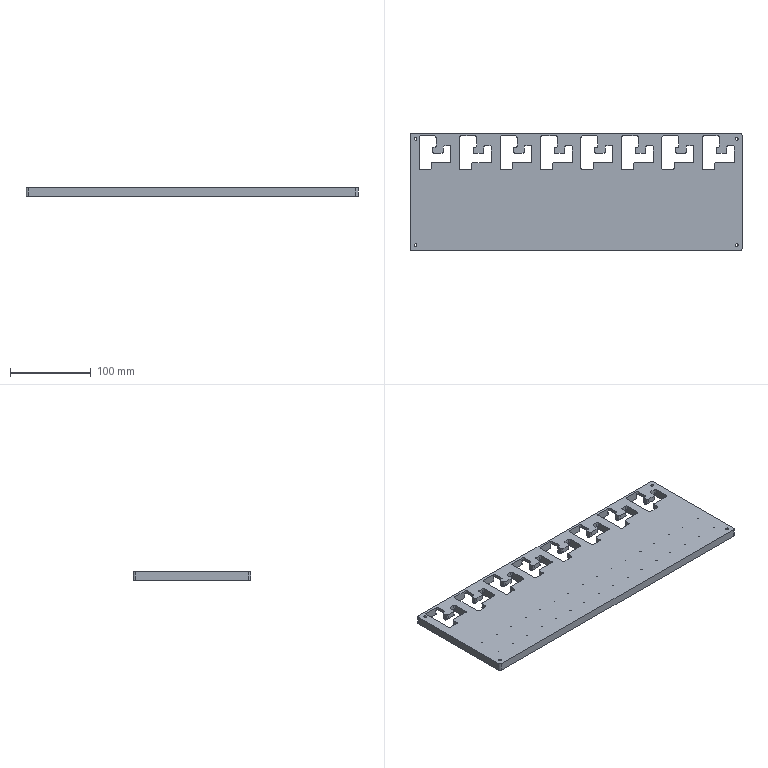NC program | NX | posted with a generic post | part box 410 x 145 x 10 mm
Lines 27 to 1051 of 104733:
(ZLEVEL_PROFILE , TOOL : D10)
N52 T10 M6
N54 G54
N56 G17 G0 G90 X199.265 Y79.6 S9500 M3
N58 G43 Z30. H10
N60 Z-1.
N62 G94 G1 X200.135 Y78.097 F2500.
N64 G3 X201.002 Y77.599 R1.
N66 G1 X201.773 Y77.6
N68 X202.5
N70 G2 X210.1 Y70. R7.6
N72 G1 Y-70.
N74 G2 X202.5 Y-77.6 R7.6
N76 G1 X201.773
N78 X201.002 Y-77.599
N80 G3 X200.135 Y-78.097 R1.
N82 G1 X199.265 Y-79.6
N84 G0 Z-2.
N86 G1 X200.135 Y-78.098
N88 G2 X201.002 Y-77.599 R1.
N90 G1 X201.773 Y-77.6
N92 X202.5
N94 G3 X210.1 Y-70. R7.6
N96 G1 Y70.
N98 G3 X202.5 Y77.6 R7.6
N100 G1 X201.773
N102 X201.002 Y77.599
N104 G2 X200.135 Y78.098 R1.
N106 G1 X199.265 Y79.6
N108 G0 Z-3.
N110 G1 X200.135 Y78.098
N112 G3 X201.002 Y77.599 R1.
N114 G1 X201.773 Y77.6
N116 X202.5
N118 G2 X210.1 Y70. R7.6
N120 G1 Y-70.
N122 G2 X202.5 Y-77.6 R7.6
N124 G1 X201.773
N126 X201.002 Y-77.599
N128 G3 X200.135 Y-78.098 R1.
N130 G1 X199.265 Y-79.6
N132 G0 Z-4.
N134 G1 X200.135 Y-78.098
N136 G2 X201.002 Y-77.599 R1.
N138 G1 X201.773 Y-77.6
N140 X202.5
N142 G3 X210.1 Y-70. R7.6
N144 G1 Y70.
N146 G3 X202.5 Y77.6 R7.6
N148 G1 X201.773
N150 X201.002 Y77.599
N152 G2 X200.135 Y78.098 R1.
N154 G1 X199.265 Y79.6
N156 G0 Z-5.
N158 G1 X200.135 Y78.098
N160 G3 X201.002 Y77.599 R1.
N162 G1 X201.773 Y77.6
N164 X202.5
N166 G2 X210.1 Y70. R7.6
N168 G1 Y-70.
N170 G2 X202.5 Y-77.6 R7.6
N172 G1 X201.773
N174 X201.002 Y-77.599
N176 G3 X200.135 Y-78.098 R1.
N178 G1 X199.265 Y-79.6
N180 G0 X199.266 Z-6.
N182 G1 X200.135 Y-78.098
N184 G2 X201.002 Y-77.599 R1.
N186 G1 X201.773 Y-77.6
N188 X202.5
N190 G3 X210.1 Y-70. R7.6
N192 G1 Y70.
N194 G3 X202.5 Y77.6 R7.6
N196 G1 X201.773
N198 X201.002 Y77.599
N200 G2 X200.135 Y78.098 R1.
N202 G1 X199.266 Y79.6
N204 G0 Z-7.
N206 G1 X200.135 Y78.098
N208 G3 X201.002 Y77.599 R1.
N210 G1 X201.773 Y77.6
N212 X202.5
N214 G2 X210.1 Y70. R7.6
N216 G1 Y-70.
N218 G2 X202.5 Y-77.6 R7.6
N220 G1 X201.773
N222 X201.002 Y-77.599
N224 G3 X200.135 Y-78.098 R1.
N226 G1 X199.266 Y-79.6
N228 G0 Z-8.
N230 G1 X200.135 Y-78.098
N232 G2 X201.002 Y-77.599 R1.
N234 G1 X201.773 Y-77.6
N236 X202.5
N238 G3 X210.1 Y-70. R7.6
N240 G1 Y70.
N242 G3 X202.5 Y77.6 R7.6
N244 G1 X201.773
N246 X201.002 Y77.599
N248 G2 X200.135 Y78.098 R1.
N250 G1 X199.266 Y79.6
N252 G0 Z-9.
N254 G1 X200.135 Y78.098
N256 G3 X201.002 Y77.599 R1.
N258 G1 X201.773 Y77.6
N260 X202.5
N262 G2 X210.1 Y70. R7.6
N264 G1 Y-70.
N266 G2 X202.5 Y-77.6 R7.6
N268 G1 X201.773
N270 X201.002 Y-77.599
N272 G3 X200.135 Y-78.098 R1.
N274 G1 X199.266 Y-79.6
N276 G0 X199.267 Z-10.
N278 G1 X200.135 Y-78.099
N280 G2 X201.002 Y-77.599 R1.
N282 G1 X201.773 Y-77.6
N284 X202.5
N286 G3 X210.1 Y-70. R7.6
N288 G1 Y70.
N290 G3 X202.5 Y77.6 R7.6
N292 G1 X201.773
N294 X201.002 Y77.599
N296 G2 X200.135 Y78.099 R1.
N298 G1 X199.267 Y79.6
N300 G0 Z30.
N302 X-199.203 Y-79.6
N304 Z-1.
N306 G1 X-200.074 Y-78.097
N308 G3 X-200.941 Y-77.599 R1.
N310 G1 X-201.715 Y-77.6
N312 X-202.5
N314 G2 X-210.1 Y-70. R7.6
N316 G1 Y70.
N318 G2 X-202.5 Y77.6 R7.6
N320 G1 X-201.715
N322 X-200.941 Y77.599
N324 G3 X-200.074 Y78.097 R1.
N326 G1 X-199.203 Y79.6
N328 G0 Z-2.
N330 G1 X-200.074 Y78.098
N332 G2 X-200.941 Y77.599 R1.
N334 G1 X-201.715 Y77.6
N336 X-202.5
N338 G3 X-210.1 Y70. R7.6
N340 G1 Y-70.
N342 G3 X-202.5 Y-77.6 R7.6
N344 G1 X-201.715
N346 X-200.941 Y-77.599
N348 G2 X-200.074 Y-78.098 R1.
N350 G1 X-199.203 Y-79.6
N352 G0 X-199.204 Z-3.
N354 G1 X-200.074 Y-78.098
N356 G3 X-200.941 Y-77.599 R1.
N358 G1 X-201.715 Y-77.6
N360 X-202.5
N362 G2 X-210.1 Y-70. R7.6
N364 G1 Y70.
N366 G2 X-202.5 Y77.6 R7.6
N368 G1 X-201.715
N370 X-200.941 Y77.599
N372 G3 X-200.074 Y78.098 R1.
N374 G1 X-199.204 Y79.6
N376 G0 Z-4.
N378 G1 X-200.074 Y78.098
N380 G2 X-200.941 Y77.599 R1.
N382 G1 X-201.715 Y77.6
N384 X-202.5
N386 G3 X-210.1 Y70. R7.6
N388 G1 Y-70.
N390 G3 X-202.5 Y-77.6 R7.6
N392 G1 X-201.715
N394 X-200.941 Y-77.599
N396 G2 X-200.074 Y-78.098 R1.
N398 G1 X-199.204 Y-79.6
N400 G0 Z-5.
N402 G1 X-200.074 Y-78.098
N404 G3 X-200.941 Y-77.599 R1.
N406 G1 X-201.715 Y-77.6
N408 X-202.5
N410 G2 X-210.1 Y-70. R7.6
N412 G1 Y70.
N414 G2 X-202.5 Y77.6 R7.6
N416 G1 X-201.715
N418 X-200.941 Y77.599
N420 G3 X-200.074 Y78.098 R1.
N422 G1 X-199.204 Y79.6
N424 G0 Z-6.
N426 G1 X-200.074 Y78.098
N428 G2 X-200.941 Y77.599 R1.
N430 G1 X-201.715 Y77.6
N432 X-202.5
N434 G3 X-210.1 Y70. R7.6
N436 G1 Y-70.
N438 G3 X-202.5 Y-77.6 R7.6
N440 G1 X-201.715
N442 X-200.941 Y-77.599
N444 G2 X-200.074 Y-78.098 R1.
N446 G1 X-199.204 Y-79.6
N448 G0 X-199.205 Z-7.
N450 G1 X-200.074 Y-78.098
N452 G3 X-200.941 Y-77.599 R1.
N454 G1 X-201.715 Y-77.6
N456 X-202.5
N458 G2 X-210.1 Y-70. R7.6
N460 G1 Y70.
N462 G2 X-202.5 Y77.6 R7.6
N464 G1 X-201.715
N466 X-200.941 Y77.599
N468 G3 X-200.074 Y78.098 R1.
N470 G1 X-199.205 Y79.6
N472 G0 Z-8.
N474 G1 X-200.074 Y78.098
N476 G2 X-200.941 Y77.599 R1.
N478 G1 X-201.715 Y77.6
N480 X-202.5
N482 G3 X-210.1 Y70. R7.6
N484 G1 Y-70.
N486 G3 X-202.5 Y-77.6 R7.6
N488 G1 X-201.715
N490 X-200.941 Y-77.599
N492 G2 X-200.074 Y-78.098 R1.
N494 G1 X-199.205 Y-79.6
N496 G0 Z-9.
N498 G1 X-200.074 Y-78.098
N500 G3 X-200.941 Y-77.599 R1.
N502 G1 X-201.715 Y-77.6
N504 X-202.5
N506 G2 X-210.1 Y-70. R7.6
N508 G1 Y70.
N510 G2 X-202.5 Y77.6 R7.6
N512 G1 X-201.715
N514 X-200.941 Y77.599
N516 G3 X-200.074 Y78.098 R1.
N518 G1 X-199.205 Y79.6
N520 G0 Z-10.
N522 G1 X-200.074 Y78.099
N524 G2 X-200.941 Y77.599 R1.
N526 G1 X-201.715 Y77.6
N528 X-202.5
N530 G3 X-210.1 Y70. R7.6
N532 G1 Y-70.
N534 G3 X-202.5 Y-77.6 R7.6
N536 G1 X-201.715
N538 X-200.941 Y-77.599
N540 G2 X-200.074 Y-78.099 R1.
N542 G1 X-199.205 Y-79.6
N544 G0 Z30.
(ZLEVEL_PROFILE_COPY , TOOL : D10)
N546 X199.351 Y79.5
N548 Z-8.
N550 G1 Z-10. F1000.
N552 X200.219 Y77.999
N554 G3 X201.086 Y77.499 R1.
N556 G1 X201.847 Y77.5
N558 X202.5
N560 G2 X210. Y70. R7.5
N562 G1 Y-70.
N564 G2 X202.5 Y-77.5 R7.5
N566 G1 X201.847
N568 X201.086 Y-77.499
N570 G3 X200.219 Y-77.999 R1.
N572 G1 X199.351 Y-79.5
N574 Z-8.
N576 G0 Z30.
N578 X-199.351
N580 Z-8.
N582 G1 Z-10.
N584 X-200.219 Y-77.999
N586 G3 X-201.086 Y-77.499 R1.
N588 G1 X-201.847 Y-77.5
N590 X-202.5
N592 G2 X-210. Y-70. R7.5
N594 G1 Y70.
N596 G2 X-202.5 Y77.5 R7.5
N598 G1 X-201.847
N600 X-201.086 Y77.499
N602 G3 X-200.219 Y77.999 R1.
N604 G1 X-199.351 Y79.5
N606 Z-8.
N608 G0 Z30.
(CAVITY_MILL , TOOL : D10)
N610 X188.147 Y-79.497
N612 Z0.55
N614 G1 Z-0.95
N616 X184.683 Y-73.497
N618 G3 X183.817 Y-72.997 R1.
N620 G1 X181.315 Y-57.505
N622 G3 X179.749 Y-47.809 R6.95
N624 G1 X178.458 Y-39.822
N626 Y48.836 F3000.
N628 G2 X176.65 Y50.661 R18.7
N630 G1 X174.876
N632 G2 X173.258 Y49.029 R18.7
N634 G1 Y-39.753
N636 G2 X178.458 Y-39.822 R13.9
N638 G1 X184.458
N640 Y51.88
N642 G2 X179.732 Y56.661 R12.7
N644 G1 X171.824
N646 G2 X167.258 Y52.042 R12.7
N648 G1 Y-58.139
N650 X169.325
N652 G2 X180.566 Y-59.646 R-7.9
N654 G1 X179.824 Y-58.703
N656 G2 X170.414 Y-57.588 R6.7
N658 X179.824 Y-58.703 R-6.7
N660 G1 X180.566 Y-59.646
N662 G2 X183.817 Y-62.109 R12.85
N664 X184.458 Y-61.484 R12.85
N666 G1 Y-39.822
N668 X190.458
N670 Y56.189
N672 G2 X184.109 Y62.661 R6.7
N674 G1 X167.502 Y62.66
N676 G2 X161.258 Y56.298 R6.7
N678 G1 Y-64.139
N680 X174.529
N682 G2 X181.379 Y-70.989 R6.85
N684 G1 Y-71.5
N686 G2 X176.396 Y-77.497 R6.1
N688 G1 X179.441
N690 G3 X182.424 Y-72.997 R7.3
N692 G1 X185.211
N694 G3 X188.193 Y-77.497 R7.3
N696 G1 X191.238
N698 G2 X186.256 Y-71.5 R6.1
N700 G1 Y-70.989
N702 G2 X190.982 Y-64.476 R6.85
N704 X190.458 Y-62.003 R6.1
N706 G1 Y-39.822
N708 G3 X189.958 Y-38.956 R1.
N710 G1 Z0.55
N712 G0 Z30.
N714 X188.147 Y-79.497
N716 Z-0.4
N718 G1 Z-1.9 F1000.
N720 X184.683 Y-73.497
N722 G3 X183.817 Y-72.997 R1.
N724 G1 X181.315 Y-57.505
N726 G3 X179.749 Y-47.809 R6.95
N728 G1 X178.458 Y-39.822
N730 Y48.836 F3000.
N732 G2 X176.65 Y50.661 R18.7
N734 G1 X174.876
N736 G2 X173.258 Y49.029 R18.7
N738 G1 Y-39.753
N740 G2 X178.458 Y-39.822 R13.9
N742 G1 X184.458
N744 Y51.88
N746 G2 X179.732 Y56.661 R12.7
N748 G1 X171.824
N750 G2 X167.258 Y52.042 R12.7
N752 G1 Y-58.139
N754 X169.325
N756 G2 X180.566 Y-59.646 R-7.9
N758 G1 X179.824 Y-58.703
N760 G2 X170.414 Y-57.588 R6.7
N762 X179.824 Y-58.703 R-6.7
N764 G1 X180.566 Y-59.646
N766 G2 X183.817 Y-62.109 R12.85
N768 X184.458 Y-61.484 R12.85
N770 G1 Y-39.822
N772 X190.458
N774 Y56.189
N776 G2 X184.109 Y62.661 R6.7
N778 G1 X167.502 Y62.66
N780 G2 X161.258 Y56.298 R6.7
N782 G1 Y-64.139
N784 X174.529
N786 G2 X181.379 Y-70.989 R6.85
N788 G1 Y-71.5
N790 G2 X176.394 Y-77.497 R6.1
N792 G1 X179.441
N794 G3 X182.424 Y-72.997 R7.3
N796 G1 X185.211
N798 G3 X188.193 Y-77.497 R7.3
N800 G1 X191.24
N802 G2 X186.256 Y-71.5 R6.1
N804 G1 Y-70.989
N806 G2 X190.982 Y-64.476 R6.85
N808 X190.458 Y-62.003 R6.1
N810 G1 Y-39.822
N812 G3 X189.958 Y-38.956 R1.
N814 G1 Z-0.4
N816 G0 X174.483 Y59.066
N818 G1 X172.328 Z-0.513 F1000.
N820 Y49.7 Z-1.004
N822 X172.393 Y49.555 Z-1.012
N824 X172.909 Y49.79 Z-1.042
N826 X174.039 Y50.035 Z-1.102
N828 X178.106 Z-1.316
N830 X179.309 Y49.765 Z-1.38
N832 X180.42 Y49.228 Z-1.445
N834 X180.864 Y48.875 Z-1.475
N836 X180.897 Y48.889 Z-1.476
N838 X180.502 Y49.364 Z-1.509
N840 X179.776 Y50.783 Z-1.592
N842 X179.425 Y52.337 Z-1.676
N844 Y59.066 Z-2.028
N846 X172.328 Z-2.4
N848 Y54.304 Z-2.65
N850 Y49.7 F3000.
N852 X172.393 Y49.555
N854 G2 X174.606 Y50.035 R5.35
N856 G1 X177.539
N858 G2 X180.864 Y48.875 R5.35
N860 G1 X180.897 Y48.889
N862 G2 X179.425 Y52.955 R6.35
N864 G1 Y59.066
N866 X172.328
N868 Y54.304
N870 G3 X172.828 Y53.438 R1.
N872 G1 Z-1.15
N874 G0 X174.483 Y59.066
N876 G1 X172.328 Z-1.263 F1000.
N878 Y49.7 Z-1.754
N880 X172.393 Y49.555 Z-1.762
N882 X172.91 Y49.79 Z-1.792
N884 X174.039 Y50.035 Z-1.852
N886 X178.106 Z-2.066
N888 X179.309 Y49.765 Z-2.13
N890 X180.42 Y49.228 Z-2.195
N892 X180.864 Y48.875 Z-2.225
N894 X180.897 Y48.889 Z-2.226
N896 X180.502 Y49.364 Z-2.259
N898 X179.776 Y50.783 Z-2.342
N900 X179.425 Y52.337 Z-2.426
N902 Y59.066 Z-2.778
N904 X172.328 Z-3.15
N906 Y54.304 Z-3.4
N908 Y49.7 F3000.
N910 X172.393 Y49.555
N912 G2 X174.606 Y50.035 R5.35
N914 G1 X177.539
N916 G2 X180.864 Y48.875 R5.35
N918 G1 X180.897 Y48.889
N920 G2 X179.425 Y52.955 R6.35
N922 G1 Y59.066
N924 X172.328
N926 Y54.304
N928 G3 X172.828 Y53.438 R1.
N930 G1 Z-1.9
N932 G0 X172.328 Y58.359
N934 G1 Y49.7 Z-2.354 F1000.
N936 X172.393 Y49.555 Z-2.362
N938 X172.91 Y49.79 Z-2.392
N940 X174.039 Y50.035 Z-2.452
N942 X178.106 Z-2.666
N944 X179.309 Y49.765 Z-2.73
N946 X180.42 Y49.228 Z-2.795
N948 X180.864 Y48.875 Z-2.825
N950 X180.897 Y48.889 Z-2.826
N952 X180.502 Y49.364 Z-2.859
N954 X179.776 Y50.783 Z-2.942
N956 X179.425 Y52.337 Z-3.026
N958 Y59.066 Z-3.378
N960 X172.328 Z-3.75
N962 Y54.304 Z-4.
N964 Y49.7 F3000.
N966 X172.393 Y49.555
N968 G2 X174.606 Y50.035 R5.35
N970 G1 X177.539
N972 G2 X180.864 Y48.875 R5.35
N974 G1 X180.897 Y48.889
N976 G2 X179.425 Y52.955 R6.35
N978 G1 Y59.066
N980 X172.328
N982 Y54.304
N984 G3 X172.828 Y53.438 R1.
N986 G1 Z-2.5
N988 G0 Z30.
N990 X179.291 Y24.546
N992 Z-0.4
N994 G1 X179.226 Y24.631 Z-0.406 F1000.
N996 X178.93 Y25.2 Z-0.439
N998 X178.409 Y25.09 Z-0.467
N1000 X175.604 Z-0.614
N1002 X174.732 Y25.262 Z-0.661
N1004 X174.22 Y25.473 Z-0.69
N1006 X174.053 Y24.878 Z-0.722
N1008 X173.463 Y23.723 Z-0.79
N1010 X172.695 Y22.755 Z-0.855
N1012 X172.281 Y22.363 Z-0.885
N1014 X171.777 Y22.005 Z-0.917
N1016 Y15.867 Z-1.239
N1018 X181.163 Z-1.731
N1020 Y22.694 Z-2.088
N1022 X180.632 Y23.054 Z-2.122
N1024 X179.868 Y23.788 Z-2.178
N1026 X179.226 Y24.631 Z-2.233
N1028 X178.93 Y25.2 Z-2.267
N1030 X178.409 Y25.09 Z-2.295
N1032 X175.604 Z-2.442
N1034 X174.732 Y25.262 Z-2.488
N1036 X174.22 Y25.473 Z-2.517
N1038 X174.053 Y24.878 Z-2.55
N1040 X173.463 Y23.723 Z-2.618
N1042 X173.079 Y23.239 Z-2.65
N1044 X176.604 Y20.441
N1046 X176.545 Y20.367 F3000.
N1048 X176.663
N1050 Y20.516
N1052 X176.604 Y20.441
N1054 X173.079 Y23.239
N1056 G2 X171.777 Y22.005 R6.35
N1058 G1 Y15.867
N1060 X181.163
N1062 Y22.694
N1064 G2 X178.93 Y25.2 R6.85
N1066 X177.876 Y25.09 R5.1
N1068 G1 X176.158
N1070 G2 X174.22 Y25.473 R5.1
N1072 X173.079 Y23.239 R6.35
N1074 G3 X172.933 Y22.25 R1.
N1076 G1 Z-1.15
N1078 G0 X179.291 Y24.546
N1080 G1 X179.226 Y24.631 Z-1.156 F1000.
N1082 X178.93 Y25.2 Z-1.189
N1084 X178.409 Y25.09 Z-1.217
N1086 X175.604 Z-1.364
N1088 X174.732 Y25.262 Z-1.411
N1090 X174.22 Y25.473 Z-1.44
N1092 X174.053 Y24.878 Z-1.472
N1094 X173.463 Y23.723 Z-1.54
N1096 X172.695 Y22.755 Z-1.605
N1098 X172.281 Y22.363 Z-1.635
N1100 X171.777 Y22.005 Z-1.667
N1102 Y15.867 Z-1.989
N1104 X181.163 Z-2.481
N1106 Y22.694 Z-2.838
N1108 X180.632 Y23.054 Z-2.872
N1110 X179.868 Y23.788 Z-2.928
N1112 X179.226 Y24.631 Z-2.983
N1114 X178.93 Y25.2 Z-3.017
N1116 X178.409 Y25.09 Z-3.045
N1118 X175.604 Z-3.192
N1120 X174.732 Y25.262 Z-3.238
N1122 X174.22 Y25.473 Z-3.267
N1124 X174.053 Y24.878 Z-3.3
N1126 X173.463 Y23.723 Z-3.368
N1128 X173.079 Y23.239 Z-3.4
N1130 X176.604 Y20.441
N1132 X176.545 Y20.367 F3000.
N1134 X176.663
N1136 Y20.516
N1138 X176.604 Y20.441
N1140 X173.079 Y23.239
N1142 G2 X171.777 Y22.005 R6.35
N1144 G1 Y15.867
N1146 X181.163
N1148 Y22.694
N1150 G2 X178.93 Y25.2 R6.85
N1152 X177.876 Y25.09 R5.1
N1154 G1 X176.158
N1156 G2 X174.22 Y25.473 R5.1
N1158 X173.079 Y23.239 R6.35
N1160 G3 X172.933 Y22.25 R1.
N1162 G1 Z-1.9
N1164 G0 X176.828 Y25.09
N1166 G1 X175.604 Z-1.964 F1000.
N1168 X174.732 Y25.262 Z-2.011
N1170 X174.22 Y25.473 Z-2.04
N1172 X174.053 Y24.878 Z-2.072
N1174 X173.463 Y23.723 Z-2.14
N1176 X172.695 Y22.755 Z-2.205
N1178 X172.281 Y22.363 Z-2.235
N1180 X171.777 Y22.005 Z-2.267
N1182 Y15.867 Z-2.589
N1184 X181.163 Z-3.081
N1186 Y22.694 Z-3.438
N1188 X180.632 Y23.054 Z-3.472
N1190 X179.868 Y23.788 Z-3.528
N1192 X179.226 Y24.631 Z-3.583
N1194 X178.93 Y25.2 Z-3.617
N1196 X178.409 Y25.09 Z-3.645
N1198 X175.604 Z-3.792
N1200 X174.732 Y25.262 Z-3.838
N1202 X174.22 Y25.473 Z-3.867
N1204 X174.053 Y24.878 Z-3.9
N1206 X173.463 Y23.723 Z-3.968
N1208 X173.079 Y23.239 Z-4.
N1210 X176.604 Y20.441
N1212 X176.545 Y20.367 F3000.
N1214 X176.663
N1216 Y20.516
N1218 X176.604 Y20.441
N1220 X173.079 Y23.239
N1222 G2 X171.777 Y22.005 R6.35
N1224 G1 Y15.867
N1226 X181.163
N1228 Y22.694
N1230 G2 X178.93 Y25.2 R6.85
N1232 X177.876 Y25.09 R5.1
N1234 G1 X176.158
N1236 G2 X174.22 Y25.473 R5.1
N1238 X173.079 Y23.239 R6.35
N1240 G3 X172.933 Y22.25 R1.
N1242 G1 Z-2.5
N1244 G0 Z30.
N1246 X167.258 Y-1.973
N1248 Z-0.4
N1250 G1 Y-13.346 Z-0.996 F1000.
N1252 X167.778 Y-12.637 Z-1.042
N1254 X169.23 Y-11.171 Z-1.15
N1256 X170.898 Y-9.956 Z-1.258
N1258 X172.738 Y-9.023 Z-1.366
N1260 X174.704 Y-8.396 Z-1.475
N1262 X176.745 Y-8.091 Z-1.583
N1264 X177.623 Z-1.629
N1266 X183.067 Z-1.914
N1268 Y-1.954 Z-2.236
N1270 X175.163 Z-2.65
N1272 X167.258 F3000.
N1274 Y-13.346
N1276 G2 X177.623 Y-8.091 R12.85
N1278 G1 X183.067
N1280 Y-1.954
N1282 X175.163
N1284 Y4.046
N1286 X161.258
N1288 Y-39.453
N1290 X167.258
N1292 Y-48.798
N1294 G2 X173.103 Y-43.886 R8.05
N1296 G1 X173.347 Y-45.061
N1298 G2 X174.741 Y-44.918 R6.85
N1300 G1 X182.404
N1302 G2 X188.754 Y-51.268 R6.35
N1304 G1 Y-56.66
N1306 G2 X181.904 Y-63.51 R6.85
N1308 G1 X178.889
N1310 G2 X173.093 Y-60.311 R6.85
N1312 X167.891 Y-54.065 R6.35
N1314 G1 Y-51.768
N1316 G2 X173.347 Y-45.061 R6.85
N1318 G1 X173.103 Y-43.886
N1320 G2 X167.258 Y-39.453 R12.85
N1322 G1 X161.258
N1324 Y-56.937
N1326 X167.258
N1328 Y-58.139
N1330 X167.884
N1332 G2 X167.258 Y-56.937 R7.55
N1334 G1 X161.258
N1336 Y-64.139
N1338 X174.529
N1340 G2 X181.379 Y-70.989 R6.85
N1342 G1 Y-71.5
N1344 G2 X176.393 Y-77.497 R6.1
N1346 G1 X179.441
N1348 G3 X182.423 Y-72.997 R7.3
N1350 G1 X185.211
N1352 G3 X188.194 Y-77.497 R7.3
N1354 G1 X191.242
N1356 G2 X186.256 Y-71.5 R6.1
N1358 G1 Y-70.989
N1360 G2 X190.982 Y-64.476 R6.85
N1362 X190.458 Y-62.003 R6.1
N1364 G1 Y-38.708
N1366 X177.623
N1368 G2 X170.773 Y-31.858 R6.85
N1370 G1 Y-20.941
N1372 G2 X177.623 Y-14.091 R6.85
N1374 G1 X189.067
N1376 Y4.046
N1378 X175.163
N1380 G3 X174.297 Y3.546 R1.
N1382 G1 Z-1.15
N1384 G0 X167.258 Y-1.973
N1386 G1 Y-13.346 Z-1.746 F1000.
N1388 X167.778 Y-12.637 Z-1.792
N1390 X169.23 Y-11.171 Z-1.9
N1392 X170.898 Y-9.956 Z-2.008
N1394 X172.738 Y-9.023 Z-2.116
N1396 X174.704 Y-8.396 Z-2.225
N1398 X176.745 Y-8.091 Z-2.333
N1400 X183.067 Z-2.664
N1402 Y-1.954 Z-2.986
N1404 X175.163 Z-3.4
N1406 X167.258 F3000.
N1408 Y-13.346
N1410 G2 X177.623 Y-8.091 R12.85
N1412 G1 X183.067
N1414 Y-1.954
N1416 X175.163
N1418 Y4.046
N1420 X161.258
N1422 Y-39.453
N1424 X167.258
N1426 Y-48.798
N1428 G2 X173.103 Y-43.886 R8.05
N1430 G1 X173.347 Y-45.061
N1432 G2 X174.741 Y-44.918 R6.85
N1434 G1 X182.404
N1436 G2 X188.754 Y-51.268 R6.35
N1438 G1 Y-56.66
N1440 G2 X181.904 Y-63.51 R6.85
N1442 G1 X178.889
N1444 G2 X173.093 Y-60.311 R6.85
N1446 X167.891 Y-54.065 R6.35
N1448 G1 Y-51.768
N1450 G2 X173.347 Y-45.061 R6.85
N1452 G1 X173.103 Y-43.886
N1454 G2 X167.258 Y-39.453 R12.85
N1456 G1 X161.258
N1458 Y-56.937
N1460 X167.258
N1462 Y-58.139
N1464 X167.884
N1466 G2 X167.258 Y-56.937 R7.55
N1468 G1 X161.258
N1470 Y-64.139
N1472 X174.529
N1474 G2 X181.379 Y-70.989 R6.85
N1476 G1 Y-71.5
N1478 G2 X176.391 Y-77.498 R6.1
N1480 G1 X179.44
N1482 G3 X182.423 Y-72.998 R7.3
N1484 G1 X185.211
N1486 G3 X188.194 Y-77.498 R7.3
N1488 G1 X191.243
N1490 G2 X186.256 Y-71.5 R6.1
N1492 G1 Y-70.989
N1494 G2 X190.982 Y-64.476 R6.85
N1496 X190.458 Y-62.003 R6.1
N1498 G1 Y-38.708
N1500 X177.623
N1502 G2 X170.773 Y-31.858 R6.85
N1504 G1 Y-20.941
N1506 G2 X177.623 Y-14.091 R6.85
N1508 G1 X189.067
N1510 Y4.046
N1512 X175.163
N1514 G3 X174.297 Y3.546 R1.
N1516 G1 Z-1.9
N1518 G0 X167.258 Y-4.834
N1520 G1 Y-13.346 Z-2.346 F1000.
N1522 X167.778 Y-12.637 Z-2.392
N1524 X169.486 Y-10.957 Z-2.518
N1526 X171.477 Y-9.622 Z-2.643
N1528 X173.074 Y-8.891 Z-2.735
N1530 X174.88 Y-8.357 Z-2.834
N1532 X176.745 Y-8.091 Z-2.933
N1534 X183.067 Z-3.264
N1536 Y-1.954 Z-3.586
N1538 X175.163 Z-4.
N1540 X167.258 F3000.
N1542 Y-13.346
N1544 G2 X177.623 Y-8.091 R12.85
N1546 G1 X183.067
N1548 Y-1.954
N1550 X175.163
N1552 Y4.046
N1554 X161.258
N1556 Y-39.453
N1558 X167.258
N1560 Y-48.798
N1562 G2 X173.103 Y-43.886 R8.05
N1564 G1 X173.347 Y-45.061
N1566 G2 X174.741 Y-44.918 R6.85
N1568 G1 X182.404
N1570 G2 X188.754 Y-51.268 R6.35
N1572 G1 Y-56.66
N1574 G2 X181.904 Y-63.51 R6.85
N1576 G1 X178.889
N1578 G2 X173.093 Y-60.311 R6.85
N1580 X167.891 Y-54.065 R6.35
N1582 G1 Y-51.768
N1584 G2 X173.347 Y-45.061 R6.85
N1586 G1 X173.103 Y-43.886
N1588 G2 X167.258 Y-39.453 R12.85
N1590 G1 X161.258
N1592 Y-56.937
N1594 X167.258
N1596 Y-58.139
N1598 X167.884
N1600 G2 X167.258 Y-56.937 R7.55
N1602 G1 X161.258
N1604 Y-64.139
N1606 X174.529
N1608 G2 X181.379 Y-70.989 R6.85
N1610 G1 Y-71.5
N1612 G2 X176.39 Y-77.498 R6.1
N1614 G1 X179.44
N1616 G3 X182.423 Y-72.998 R7.3
N1618 G1 X185.211
N1620 G3 X188.195 Y-77.498 R7.3
N1622 G1 X191.244
N1624 G2 X186.256 Y-71.5 R6.1
N1626 G1 Y-70.989
N1628 G2 X190.458 Y-64.671 R6.85
N1630 G1 Y-38.708
N1632 X177.623
N1634 G2 X170.773 Y-31.858 R6.85
N1636 G1 Y-20.941
N1638 G2 X177.623 Y-14.091 R6.85
N1640 G1 X189.067
N1642 Y4.046
N1644 X175.163
N1646 G3 X174.297 Y3.546 R1.
N1648 G1 Z-2.5
N1650 G0 Z30.
N1652 X192.522 Y-79.6
N1654 Z-3.45
N1656 G1 Z-4.95 F1000.
N1658 X192.007 Y-78.147
N1660 G3 X191.246 Y-77.498 R1.
N1662 G2 X186.256 Y-71.5 R6.1 F3000.
N1664 G1 Y-63.51
N1666 X178.889
N1668 G2 X173.093 Y-60.311 R6.85
N1670 X167.891 Y-54.065 R6.35
N1672 G1 Y-49.623
N1674 G2 X174.741 Y-42.773 R6.85
N1676 G1 X184.594
N1678 G2 X190.458 Y-46.083 R6.85
N1680 G1 Y-41.361
N1682 X172.795
N1684 G2 X165.945 Y-34.511 R6.85
N1686 G1 Y-30.456
N1688 G2 X161.258 Y-32.391 R6.85
N1690 G1 Y-64.139
N1692 X174.529
N1694 G2 X181.379 Y-70.989 R6.85
N1696 G1 Y-71.5
N1698 G2 X176.388 Y-77.498 R6.1
N1700 G3 X175.628 Y-78.147 R1.
N1702 G1 X175.113 Y-79.6
N1704 Z-3.45
N1706 G0 X192.524 Z-4.4
N1708 G1 Z-5.9 F1000.
N1710 X192.009 Y-78.148
N1712 G3 X191.248 Y-77.499 R1.
N1714 G2 X186.256 Y-71.5 R6.1 F3000.
N1716 G1 Y-63.51
N1718 X178.889
N1720 G2 X173.093 Y-60.311 R6.85
N1722 X167.891 Y-54.065 R6.35
N1724 G1 Y-49.623
N1726 G2 X174.741 Y-42.773 R6.85
N1728 G1 X184.594
N1730 G2 X190.458 Y-46.083 R6.85
N1732 G1 Y-41.361
N1734 X172.795
N1736 G2 X165.945 Y-34.511 R6.85
N1738 G1 Y-30.456
N1740 G2 X161.258 Y-32.391 R6.85
N1742 G1 Y-64.139
N1744 X174.529
N1746 G2 X181.379 Y-70.989 R6.85
N1748 G1 Y-71.5
N1750 G2 X176.387 Y-77.499 R6.1
N1752 G3 X175.626 Y-78.148 R1.
N1754 G1 X175.11 Y-79.6
N1756 Z-4.4
N1758 G0 Z30.
N1760 X173.127 Y-41.361
N1762 Z-4.4
N1764 G1 X172.795 Z-4.417 F1000.
N1766 X172.154 Z-4.451
N1768 X170.605 Y-41.033 Z-4.534
N1770 X169.172 Y-40.359 Z-4.617
N1772 X167.931 Y-39.376 Z-4.7
N1774 X166.947 Y-38.135 Z-4.783
N1776 X166.274 Y-36.702 Z-4.866
N1778 X165.945 Y-35.153 Z-4.949
N1780 Y-34.511 Z-4.983
N1782 Y-30.456 Z-5.195
N1784 X165.485 Y-30.903 Z-5.229
N1786 X164.392 Y-31.622 Z-5.297
N1788 X163.182 Y-32.122 Z-5.366
N1790 X161.9 Y-32.383 Z-5.434
N1792 X161.258 Y-32.391 Z-5.468
N1794 Y-48.265 Z-6.3
N1796 Y-64.139 F3000.
N1798 X172.039
N1800 Y-60.021
N1802 G2 X167.891 Y-54.065 R6.35
N1804 G1 Y-49.623
N1806 G2 X174.741 Y-42.773 R6.85
N1808 G1 X184.594
N1810 G2 X190.458 Y-46.083 R6.85
N1812 G1 Y-41.361
N1814 X172.795
N1816 G2 X165.945 Y-34.511 R6.85
N1818 G1 Y-30.456
N1820 G2 X161.258 Y-32.391 R6.85
N1822 G1 Y-48.265
N1824 G3 X161.758 Y-49.131 R1.
N1826 G1 Z-4.8
N1828 G0 Z30.
N1830 X183.217 Y-41.361
N1832 Z-4.8
N1834 G1 X172.795 Z-5.346 F1000.
N1836 X172.154 Z-5.38
N1838 X170.605 Y-41.033 Z-5.463
N1840 X169.172 Y-40.359 Z-5.546
N1842 X167.931 Y-39.376 Z-5.629
N1844 X166.947 Y-38.135 Z-5.712
N1846 X166.274 Y-36.702 Z-5.795
N1848 X165.945 Y-35.153 Z-5.878
N1850 Y-34.511 Z-5.911
N1852 Y-32.391 Z-6.022
N1854 X161.258 Z-6.268
N1856 Y-48.265 Z-7.1
N1858 Y-64.139 F3000.
N1860 X172.039
N1862 Y-60.021
N1864 G2 X167.891 Y-54.065 R6.35
N1866 G1 Y-49.623
N1868 G2 X174.741 Y-42.773 R6.85
N1870 G1 X184.594
N1872 G2 X190.458 Y-46.083 R6.85
N1874 G1 Y-41.361
N1876 X172.795
N1878 G2 X165.945 Y-34.511 R6.85
N1880 G1 Y-32.391
N1882 X161.258
N1884 Y-48.265
N1886 G3 X161.758 Y-49.131 R1.
N1888 G1 Z-5.6
N1890 G0 Z30.
N1892 X183.217 Y-41.361
N1894 Z-5.6
N1896 G1 X172.795 Z-6.146 F1000.
N1898 X172.154 Z-6.18
N1900 X170.605 Y-41.033 Z-6.263
N1902 X169.172 Y-40.359 Z-6.346
N1904 X167.931 Y-39.376 Z-6.429
N1906 X166.947 Y-38.135 Z-6.512
N1908 X166.274 Y-36.702 Z-6.595
N1910 X165.945 Y-35.153 Z-6.678
N1912 Y-34.511 Z-6.711
N1914 Y-32.391 Z-6.822
N1916 X161.258 Z-7.068
N1918 Y-48.265 Z-7.9
N1920 Y-64.139 F3000.
N1922 X172.039
N1924 Y-60.021
N1926 G2 X167.891 Y-54.065 R6.35
N1928 G1 Y-49.623
N1930 G2 X174.741 Y-42.773 R6.85
N1932 G1 X184.594
N1934 G2 X190.458 Y-46.083 R6.85
N1936 G1 Y-41.361
N1938 X172.795
N1940 G2 X165.945 Y-34.511 R6.85
N1942 G1 Y-32.391
N1944 X161.258
N1946 Y-48.265
N1948 G3 X161.758 Y-49.131 R1.
N1950 G1 Z-6.4
N1952 G0 Z30.
N1954 X181.309 Y-41.361
N1956 Z-6.4
N1958 G1 X172.795 Z-6.846 F1000.
N1960 X172.154 Z-6.88
N1962 X170.605 Y-41.033 Z-6.963
N1964 X169.172 Y-40.359 Z-7.046
N1966 X167.931 Y-39.376 Z-7.129
N1968 X166.947 Y-38.135 Z-7.212
N1970 X166.274 Y-36.702 Z-7.295
N1972 X165.945 Y-35.153 Z-7.378
N1974 Y-34.511 Z-7.411
N1976 Y-32.391 Z-7.522
N1978 X161.258 Z-7.768
N1980 Y-48.265 Z-8.6
N1982 Y-64.139 F3000.
N1984 X172.039
N1986 Y-60.021
N1988 G2 X167.891 Y-54.065 R6.35
N1990 G1 Y-49.623
N1992 G2 X174.741 Y-42.773 R6.85
N1994 G1 X184.594
N1996 G2 X190.458 Y-46.083 R6.85
N1998 G1 Y-41.361
N2000 X172.795
N2002 G2 X165.945 Y-34.511 R6.85
N2004 G1 Y-32.391
N2006 X161.258
N2008 Y-48.265
N2010 G3 X161.758 Y-49.131 R1.
N2012 G1 Z-7.1
N2014 G0 Z30.
N2016 X181.309 Y-41.361
N2018 Z-7.1
N2020 G1 X172.795 Z-7.546 F1000.
N2022 X172.154 Z-7.58
N2024 X170.605 Y-41.033 Z-7.663
N2026 X169.172 Y-40.359 Z-7.746
N2028 X167.931 Y-39.376 Z-7.829
N2030 X166.947 Y-38.135 Z-7.912
N2032 X166.274 Y-36.702 Z-7.995
N2034 X165.945 Y-35.153 Z-8.078
N2036 Y-34.511 Z-8.111
N2038 Y-32.391 Z-8.222
N2040 X161.258 Z-8.468
N2042 Y-48.265 Z-9.3
N2044 Y-64.139 F3000.
N2046 X172.039
N2048 Y-60.021
N2050 G2 X167.891 Y-54.065 R6.35
N2052 G1 Y-49.623
N2054 G2 X174.741 Y-42.773 R6.85
N2056 G1 X184.594
N2058 G2 X190.458 Y-46.083 R6.85
N2060 G1 Y-41.361
N2062 X172.795
N2064 G2 X165.945 Y-34.511 R6.85
N2066 G1 Y-32.391
N2068 X161.258
N2070 Y-48.265
N2072 G3 X161.758 Y-49.131 R1.
N2074 G1 Z-7.8
N2076 G0 Z30.
N2078 X181.309 Y-41.361
N2080 Z-7.8
N2082 G1 X172.795 Z-8.246 F1000.